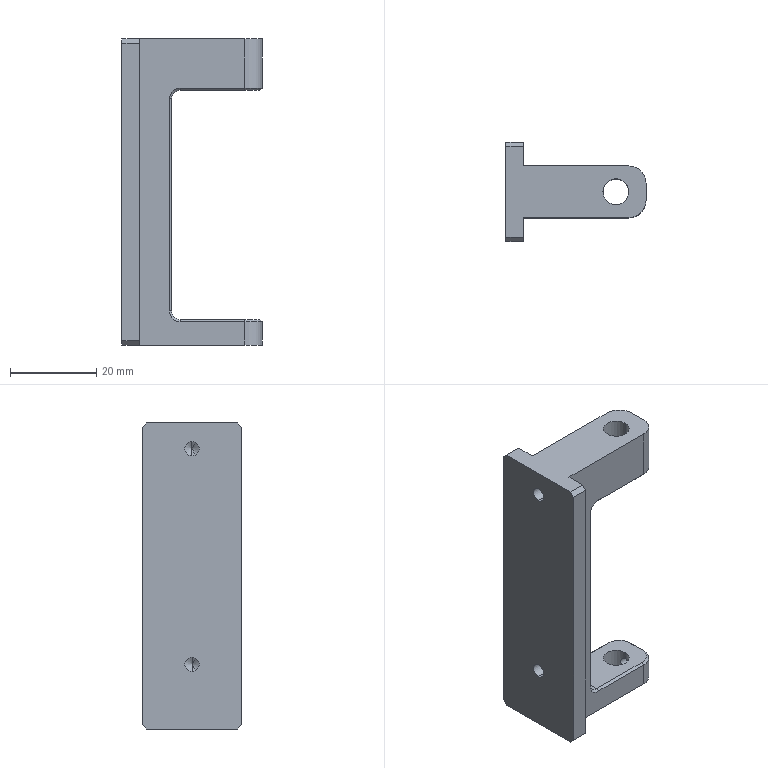Part | STEP file | 10000020470swp000-1 | 1 solid | 56 faces | box 32.5 x 23 x 71 mm | volume 16585 mm3 | plane 26 | cylinder 18 | cone 12 | commonest cylinder face diameters 2.5 x4 3.3 x4 6 x4 8 x4 4 x2